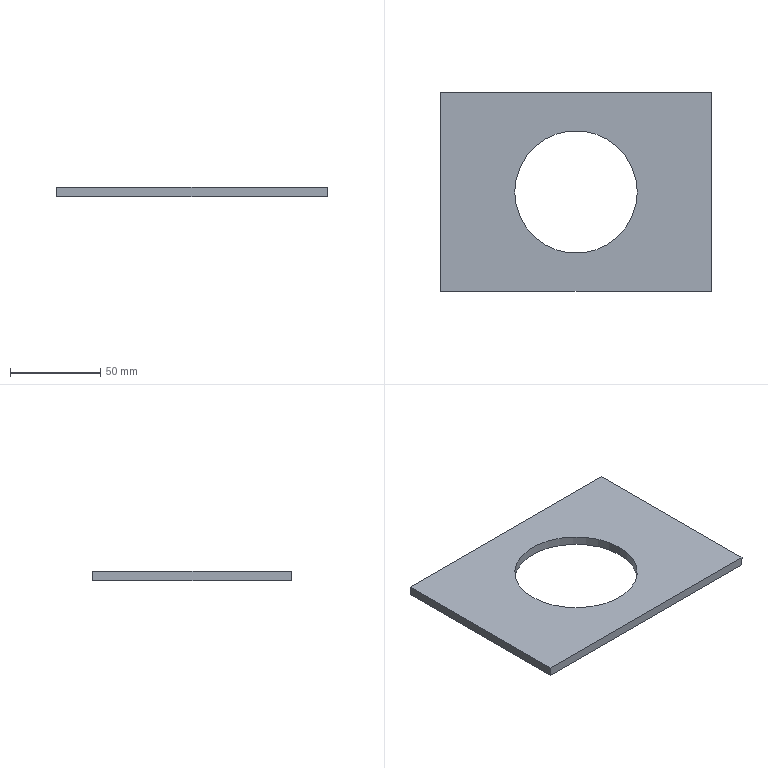Part | SolidWorks | features Cut 1, Extrusion 1 | 1 solid | 8 faces | box 150 x 110 x 5 mm | volume 64431 mm3 | plane 6 | cylinder 2 | commonest cylinder face diameters 67.832 x2
STEP:
#1=CARTESIAN_POINT('',(-33.916,0.,2.5));
#2=VERTEX_POINT('',#1);
#3=CARTESIAN_POINT('',(33.916,0.,2.5));
#4=VERTEX_POINT('',#3);
#5=CARTESIAN_POINT('',(0.,0.,2.5));
#6=DIRECTION('',(0.,0.,1.));
#7=DIRECTION('',(1.,0.,0.));
#8=AXIS2_PLACEMENT_3D('',#5,#6,#7);
#9=CIRCLE('',#8,33.916);
#10=EDGE_CURVE('',#2,#4,#9,.T.);
#11=ORIENTED_EDGE('',*,*,#10,.T.);
#12=CARTESIAN_POINT('',(33.916,0.,-2.5));
#13=VERTEX_POINT('',#12);
#14=CARTESIAN_POINT('',(33.916,0.,7.5));
#15=DIRECTION('',(0.,0.,-1.));
#16=VECTOR('',#15,1000.);
#17=LINE('',#14,#16);
#18=EDGE_CURVE('',#4,#13,#17,.T.);
#19=ORIENTED_EDGE('',*,*,#18,.T.);
#20=CARTESIAN_POINT('',(-33.916,0.,-2.5));
#21=VERTEX_POINT('',#20);
#22=CARTESIAN_POINT('',(0.,0.,-2.5));
#23=DIRECTION('',(0.,0.,-1.));
#24=DIRECTION('',(-1.,0.,0.));
#25=AXIS2_PLACEMENT_3D('',#22,#23,#24);
#26=CIRCLE('',#25,33.916);
#27=EDGE_CURVE('',#13,#21,#26,.T.);
#28=ORIENTED_EDGE('',*,*,#27,.T.);
#29=CARTESIAN_POINT('',(-33.916,0.,7.5));
#30=DIRECTION('',(0.,0.,-1.));
#31=VECTOR('',#30,1000.);
#32=LINE('',#29,#31);
#33=EDGE_CURVE('',#2,#21,#32,.T.);
#34=ORIENTED_EDGE('',*,*,#33,.F.);
#35=EDGE_LOOP('',(#11,#19,#28,#34));
#36=FACE_OUTER_BOUND('',#35,.T.);
#37=CARTESIAN_POINT('',(0.,0.,7.5));
#38=DIRECTION('',(0.,0.,-1.));
#39=DIRECTION('',(-1.,0.,0.));
#40=AXIS2_PLACEMENT_3D('',#37,#38,#39);
#41=CYLINDRICAL_SURFACE('',#40,33.916);
#42=ADVANCED_FACE('',(#36),#41,.F.);
#43=CARTESIAN_POINT('',(-75.,55.,-2.5));
#44=VERTEX_POINT('',#43);
#45=CARTESIAN_POINT('',(-75.,-55.,-2.5));
#46=VERTEX_POINT('',#45);
#47=CARTESIAN_POINT('',(-75.,-55.,-2.5));
#48=DIRECTION('',(0.,-1.,0.));
#49=VECTOR('',#48,1000.);
#50=LINE('',#47,#49);
#51=EDGE_CURVE('',#44,#46,#50,.T.);
#52=ORIENTED_EDGE('',*,*,#51,.T.);
#53=CARTESIAN_POINT('',(-75.,-55.,2.5));
#54=VERTEX_POINT('',#53);
#55=CARTESIAN_POINT('',(-75.,-55.,2.5));
#56=DIRECTION('',(0.,0.,-1.));
#57=VECTOR('',#56,1000.);
#58=LINE('',#55,#57);
#59=EDGE_CURVE('',#54,#46,#58,.T.);
#60=ORIENTED_EDGE('',*,*,#59,.F.);
#61=CARTESIAN_POINT('',(-75.,55.,2.5));
#62=VERTEX_POINT('',#61);
#63=CARTESIAN_POINT('',(-75.,-55.,2.5));
#64=DIRECTION('',(0.,-1.,0.));
#65=VECTOR('',#64,1000.);
#66=LINE('',#63,#65);
#67=EDGE_CURVE('',#62,#54,#66,.T.);
#68=ORIENTED_EDGE('',*,*,#67,.F.);
#69=CARTESIAN_POINT('',(-75.,55.,2.5));
#70=DIRECTION('',(0.,0.,-1.));
#71=VECTOR('',#70,1000.);
#72=LINE('',#69,#71);
#73=EDGE_CURVE('',#62,#44,#72,.T.);
#74=ORIENTED_EDGE('',*,*,#73,.T.);
#75=EDGE_LOOP('',(#52,#60,#68,#74));
#76=FACE_OUTER_BOUND('',#75,.T.);
#77=CARTESIAN_POINT('',(-75.,-55.,2.5));
#78=DIRECTION('',(1.,0.,0.));
#79=DIRECTION('',(0.,0.,-1.));
#80=AXIS2_PLACEMENT_3D('',#77,#78,#79);
#81=PLANE('',#80);
#82=ADVANCED_FACE('',(#76),#81,.F.);
#83=CARTESIAN_POINT('',(75.,-55.,-2.5));
#84=VERTEX_POINT('',#83);
#85=CARTESIAN_POINT('',(75.,-55.,-2.5));
#86=DIRECTION('',(1.,0.,0.));
#87=VECTOR('',#86,1000.);
#88=LINE('',#85,#87);
#89=EDGE_CURVE('',#46,#84,#88,.T.);
#90=ORIENTED_EDGE('',*,*,#89,.T.);
#91=CARTESIAN_POINT('',(75.,-55.,2.5));
#92=VERTEX_POINT('',#91);
#93=CARTESIAN_POINT('',(75.,-55.,2.5));
#94=DIRECTION('',(0.,0.,-1.));
#95=VECTOR('',#94,1000.);
#96=LINE('',#93,#95);
#97=EDGE_CURVE('',#92,#84,#96,.T.);
#98=ORIENTED_EDGE('',*,*,#97,.F.);
#99=CARTESIAN_POINT('',(75.,-55.,2.5));
#100=DIRECTION('',(1.,0.,0.));
#101=VECTOR('',#100,1000.);
#102=LINE('',#99,#101);
#103=EDGE_CURVE('',#54,#92,#102,.T.);
#104=ORIENTED_EDGE('',*,*,#103,.F.);
#105=ORIENTED_EDGE('',*,*,#59,.T.);
#106=EDGE_LOOP('',(#90,#98,#104,#105));
#107=FACE_OUTER_BOUND('',#106,.T.);
#108=CARTESIAN_POINT('',(75.,-55.,2.5));
#109=DIRECTION('',(0.,1.,0.));
#110=DIRECTION('',(-1.,0.,0.));
#111=AXIS2_PLACEMENT_3D('',#108,#109,#110);
#112=PLANE('',#111);
#113=ADVANCED_FACE('',(#107),#112,.F.);
#114=CARTESIAN_POINT('',(75.,55.,-2.5));
#115=VERTEX_POINT('',#114);
#116=CARTESIAN_POINT('',(75.,-55.,-2.5));
#117=DIRECTION('',(0.,1.,0.));
#118=VECTOR('',#117,1000.);
#119=LINE('',#116,#118);
#120=EDGE_CURVE('',#84,#115,#119,.T.);
#121=ORIENTED_EDGE('',*,*,#120,.T.);
#122=CARTESIAN_POINT('',(75.,55.,2.5));
#123=VERTEX_POINT('',#122);
#124=CARTESIAN_POINT('',(75.,55.,2.5));
#125=DIRECTION('',(0.,0.,-1.));
#126=VECTOR('',#125,1000.);
#127=LINE('',#124,#126);
#128=EDGE_CURVE('',#123,#115,#127,.T.);
#129=ORIENTED_EDGE('',*,*,#128,.F.);
#130=CARTESIAN_POINT('',(75.,-55.,2.5));
#131=DIRECTION('',(0.,1.,0.));
#132=VECTOR('',#131,1000.);
#133=LINE('',#130,#132);
#134=EDGE_CURVE('',#92,#123,#133,.T.);
#135=ORIENTED_EDGE('',*,*,#134,.F.);
#136=ORIENTED_EDGE('',*,*,#97,.T.);
#137=EDGE_LOOP('',(#121,#129,#135,#136));
#138=FACE_OUTER_BOUND('',#137,.T.);
#139=CARTESIAN_POINT('',(75.,-55.,2.5));
#140=DIRECTION('',(-1.,0.,0.));
#141=DIRECTION('',(0.,0.,1.));
#142=AXIS2_PLACEMENT_3D('',#139,#140,#141);
#143=PLANE('',#142);
#144=ADVANCED_FACE('',(#138),#143,.F.);
#145=CARTESIAN_POINT('',(75.,55.,-2.5));
#146=DIRECTION('',(-1.,0.,0.));
#147=VECTOR('',#146,1000.);
#148=LINE('',#145,#147);
#149=EDGE_CURVE('',#115,#44,#148,.T.);
#150=ORIENTED_EDGE('',*,*,#149,.T.);
#151=ORIENTED_EDGE('',*,*,#73,.F.);
#152=CARTESIAN_POINT('',(75.,55.,2.5));
#153=DIRECTION('',(-1.,0.,0.));
#154=VECTOR('',#153,1000.);
#155=LINE('',#152,#154);
#156=EDGE_CURVE('',#123,#62,#155,.T.);
#157=ORIENTED_EDGE('',*,*,#156,.F.);
#158=ORIENTED_EDGE('',*,*,#128,.T.);
#159=EDGE_LOOP('',(#150,#151,#157,#158));
#160=FACE_OUTER_BOUND('',#159,.T.);
#161=CARTESIAN_POINT('',(75.,55.,2.5));
#162=DIRECTION('',(0.,-1.,0.));
#163=DIRECTION('',(1.,0.,0.));
#164=AXIS2_PLACEMENT_3D('',#161,#162,#163);
#165=PLANE('',#164);
#166=ADVANCED_FACE('',(#160),#165,.F.);
#167=ORIENTED_EDGE('',*,*,#10,.F.);
#168=CARTESIAN_POINT('',(0.,0.,2.5));
#169=DIRECTION('',(0.,0.,1.));
#170=DIRECTION('',(1.,0.,0.));
#171=AXIS2_PLACEMENT_3D('',#168,#169,#170);
#172=CIRCLE('',#171,33.916);
#173=EDGE_CURVE('',#4,#2,#172,.T.);
#174=ORIENTED_EDGE('',*,*,#173,.F.);
#175=EDGE_LOOP('',(#167,#174));
#176=FACE_BOUND('',#175,.T.);
#177=ORIENTED_EDGE('',*,*,#67,.T.);
#178=ORIENTED_EDGE('',*,*,#103,.T.);
#179=ORIENTED_EDGE('',*,*,#134,.T.);
#180=ORIENTED_EDGE('',*,*,#156,.T.);
#181=EDGE_LOOP('',(#177,#178,#179,#180));
#182=FACE_OUTER_BOUND('',#181,.T.);
#183=CARTESIAN_POINT('',(0.,0.,2.5));
#184=DIRECTION('',(0.,0.,1.));
#185=DIRECTION('',(1.,0.,0.));
#186=AXIS2_PLACEMENT_3D('',#183,#184,#185);
#187=PLANE('',#186);
#188=ADVANCED_FACE('',(#176,#182),#187,.T.);
#189=CARTESIAN_POINT('',(0.,0.,-2.5));
#190=DIRECTION('',(0.,0.,-1.));
#191=DIRECTION('',(-1.,0.,0.));
#192=AXIS2_PLACEMENT_3D('',#189,#190,#191);
#193=CIRCLE('',#192,33.916);
#194=EDGE_CURVE('',#21,#13,#193,.T.);
#195=ORIENTED_EDGE('',*,*,#194,.F.);
#196=ORIENTED_EDGE('',*,*,#27,.F.);
#197=EDGE_LOOP('',(#195,#196));
#198=FACE_BOUND('',#197,.T.);
#199=ORIENTED_EDGE('',*,*,#51,.F.);
#200=ORIENTED_EDGE('',*,*,#149,.F.);
#201=ORIENTED_EDGE('',*,*,#120,.F.);
#202=ORIENTED_EDGE('',*,*,#89,.F.);
#203=EDGE_LOOP('',(#199,#200,#201,#202));
#204=FACE_OUTER_BOUND('',#203,.T.);
#205=CARTESIAN_POINT('',(0.,0.,-2.5));
#206=DIRECTION('',(0.,0.,1.));
#207=DIRECTION('',(1.,0.,0.));
#208=AXIS2_PLACEMENT_3D('',#205,#206,#207);
#209=PLANE('',#208);
#210=ADVANCED_FACE('',(#198,#204),#209,.F.);
#211=ORIENTED_EDGE('',*,*,#18,.F.);
#212=ORIENTED_EDGE('',*,*,#173,.T.);
#213=ORIENTED_EDGE('',*,*,#33,.T.);
#214=ORIENTED_EDGE('',*,*,#194,.T.);
#215=EDGE_LOOP('',(#211,#212,#213,#214));
#216=FACE_OUTER_BOUND('',#215,.T.);
#217=CARTESIAN_POINT('',(0.,0.,7.5));
#218=DIRECTION('',(0.,0.,-1.));
#219=DIRECTION('',(-1.,0.,0.));
#220=AXIS2_PLACEMENT_3D('',#217,#218,#219);
#221=CYLINDRICAL_SURFACE('',#220,33.916);
#222=ADVANCED_FACE('',(#216),#221,.F.);
#223=CLOSED_SHELL('',(#42,#82,#113,#144,#166,#188,#210,#222));
#224=MANIFOLD_SOLID_BREP('',#223);
#225=CARTESIAN_POINT('',(0.,0.,0.));
#226=DIRECTION('',(0.,0.,1.));
#227=DIRECTION('',(1.,0.,0.));
#228=AXIS2_PLACEMENT_3D('',#225,#226,#227);
#229=(LENGTH_UNIT()NAMED_UNIT(*)SI_UNIT(.MILLI.,.METRE.));
#230=UNCERTAINTY_MEASURE_WITH_UNIT(LENGTH_MEASURE(0.00001),#229,'','');
#231=(NAMED_UNIT(*)PLANE_ANGLE_UNIT()SI_UNIT($,.RADIAN.));
#232=(NAMED_UNIT(*)SI_UNIT($,.STERADIAN.)SOLID_ANGLE_UNIT());
#233=(GEOMETRIC_REPRESENTATION_CONTEXT(3)GLOBAL_UNCERTAINTY_ASSIGNED_CONTEXT((#230))GLOBAL_UNIT_ASSIGNED_CONTEXT((#229,#231,#232))REPRESENTATION_CONTEXT('',''));
#234=ADVANCED_BREP_SHAPE_REPRESENTATION('',(#224,#228),#233);